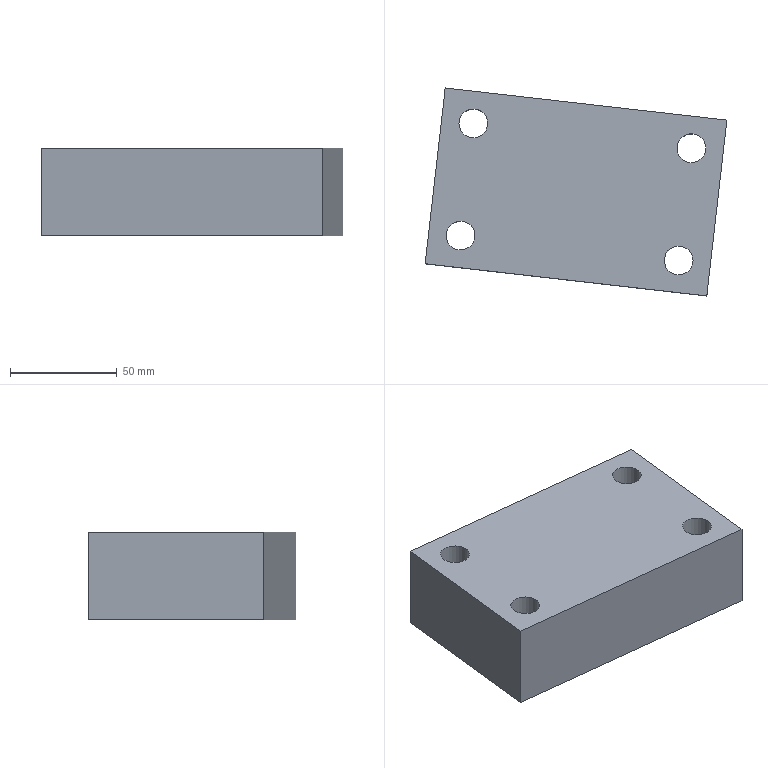Part | NX | features solid 2 | 1 solid | 18 faces | box 141.541 x 97.522 x 41 mm | volume 418863 mm3 | plane 10 | cylinder 8 | commonest cylinder face diameters 13.5 x4 20 x4
STEP:
#1=CARTESIAN_POINT('',(2413.748,-103.871,101.));
#2=VERTEX_POINT('',#1);
#3=CARTESIAN_POINT('',(2406.998,-103.871,101.));
#4=DIRECTION('',(0.,0.,-1.));
#5=DIRECTION('',(1.,0.,0.));
#6=AXIS2_PLACEMENT_3D('',#3,#4,#5);
#7=CIRCLE('',#6,6.75);
#8=EDGE_CURVE('',#2,#2,#7,.T.);
#9=ORIENTED_EDGE('',*,*,#8,.T.);
#10=EDGE_LOOP('',(#9));
#11=FACE_BOUND('',#10,.T.);
#12=CARTESIAN_POINT('',(2419.575,-52.73,101.));
#13=VERTEX_POINT('',#12);
#14=CARTESIAN_POINT('',(2412.998,-51.211,101.));
#15=DIRECTION('',(0.,0.,1.));
#16=DIRECTION('',(0.9744,-0.225,0.));
#17=AXIS2_PLACEMENT_3D('',#14,#15,#16);
#18=CIRCLE('',#17,6.75);
#19=EDGE_CURVE('',#13,#13,#18,.T.);
#20=ORIENTED_EDGE('',*,*,#19,.F.);
#21=EDGE_LOOP('',(#20));
#22=FACE_BOUND('',#21,.T.);
#23=CARTESIAN_POINT('',(2420.203,-120.472,101.));
#24=VERTEX_POINT('',#23);
#25=CARTESIAN_POINT('',(2288.058,-105.416,101.));
#26=VERTEX_POINT('',#25);
#27=CARTESIAN_POINT('',(2343.698,-111.756,101.));
#28=DIRECTION('',(-0.9936,0.1132,0.));
#29=VECTOR('',#28,1000.);
#30=LINE('',#27,#29);
#31=EDGE_CURVE('',#24,#26,#30,.T.);
#32=ORIENTED_EDGE('',*,*,#31,.F.);
#33=CARTESIAN_POINT('',(2429.599,-38.006,101.));
#34=VERTEX_POINT('',#33);
#35=CARTESIAN_POINT('',(2424.505,-82.717,101.));
#36=DIRECTION('',(-0.1132,-0.9936,0.));
#37=VECTOR('',#36,1000.);
#38=LINE('',#35,#37);
#39=EDGE_CURVE('',#34,#24,#38,.T.);
#40=ORIENTED_EDGE('',*,*,#39,.F.);
#41=CARTESIAN_POINT('',(2297.454,-22.95,101.));
#42=VERTEX_POINT('',#41);
#43=CARTESIAN_POINT('',(2353.094,-29.289,101.));
#44=DIRECTION('',(0.9936,-0.1132,0.));
#45=VECTOR('',#44,1000.);
#46=LINE('',#43,#45);
#47=EDGE_CURVE('',#42,#34,#46,.T.);
#48=ORIENTED_EDGE('',*,*,#47,.F.);
#49=CARTESIAN_POINT('',(2292.36,-67.661,101.));
#50=DIRECTION('',(0.1132,0.9936,0.));
#51=VECTOR('',#50,1000.);
#52=LINE('',#49,#51);
#53=EDGE_CURVE('',#26,#42,#52,.T.);
#54=ORIENTED_EDGE('',*,*,#53,.F.);
#55=EDGE_LOOP('',(#32,#40,#48,#54));
#56=FACE_BOUND('',#55,.T.);
#57=CARTESIAN_POINT('',(2298.083,-90.692,101.));
#58=VERTEX_POINT('',#57);
#59=CARTESIAN_POINT('',(2304.66,-92.211,101.));
#60=DIRECTION('',(0.,0.,1.));
#61=DIRECTION('',(-0.9744,0.225,0.));
#62=AXIS2_PLACEMENT_3D('',#59,#60,#61);
#63=CIRCLE('',#62,6.75);
#64=EDGE_CURVE('',#58,#58,#63,.T.);
#65=ORIENTED_EDGE('',*,*,#64,.F.);
#66=EDGE_LOOP('',(#65));
#67=FACE_BOUND('',#66,.T.);
#68=CARTESIAN_POINT('',(2303.91,-39.552,101.));
#69=VERTEX_POINT('',#68);
#70=CARTESIAN_POINT('',(2310.66,-39.552,101.));
#71=DIRECTION('',(0.,0.,-1.));
#72=DIRECTION('',(-1.,0.,0.));
#73=AXIS2_PLACEMENT_3D('',#70,#71,#72);
#74=CIRCLE('',#73,6.75);
#75=EDGE_CURVE('',#69,#69,#74,.T.);
#76=ORIENTED_EDGE('',*,*,#75,.T.);
#77=EDGE_LOOP('',(#76));
#78=FACE_BOUND('',#77,.T.);
#79=CARTESIAN_POINT('',(94.5,193.,101.));
#80=DIRECTION('',(0.,0.,1.));
#81=DIRECTION('',(-1.,0.,0.));
#82=AXIS2_PLACEMENT_3D('',#79,#80,#81);
#83=PLANE('',#82);
#84=ADVANCED_FACE('',(#11,#22,#56,#67,#78),#83,.T.);
#85=CARTESIAN_POINT('',(2416.998,-103.871,60.));
#86=VERTEX_POINT('',#85);
#87=CARTESIAN_POINT('',(2406.998,-103.871,60.));
#88=DIRECTION('',(0.,0.,1.));
#89=DIRECTION('',(1.,0.,0.));
#90=AXIS2_PLACEMENT_3D('',#87,#88,#89);
#91=CIRCLE('',#90,10.);
#92=EDGE_CURVE('',#86,#86,#91,.T.);
#93=ORIENTED_EDGE('',*,*,#92,.T.);
#94=EDGE_LOOP('',(#93));
#95=FACE_BOUND('',#94,.T.);
#96=CARTESIAN_POINT('',(2422.741,-53.461,60.));
#97=VERTEX_POINT('',#96);
#98=CARTESIAN_POINT('',(2412.998,-51.211,60.));
#99=DIRECTION('',(0.,0.,-1.));
#100=DIRECTION('',(0.9744,-0.225,0.));
#101=AXIS2_PLACEMENT_3D('',#98,#99,#100);
#102=CIRCLE('',#101,10.);
#103=EDGE_CURVE('',#97,#97,#102,.T.);
#104=ORIENTED_EDGE('',*,*,#103,.F.);
#105=EDGE_LOOP('',(#104));
#106=FACE_BOUND('',#105,.T.);
#107=CARTESIAN_POINT('',(2420.203,-120.472,60.));
#108=VERTEX_POINT('',#107);
#109=CARTESIAN_POINT('',(2429.599,-38.006,60.));
#110=VERTEX_POINT('',#109);
#111=CARTESIAN_POINT('',(2424.505,-82.717,60.));
#112=DIRECTION('',(0.1132,0.9936,0.));
#113=VECTOR('',#112,1000.);
#114=LINE('',#111,#113);
#115=EDGE_CURVE('',#108,#110,#114,.T.);
#116=ORIENTED_EDGE('',*,*,#115,.F.);
#117=CARTESIAN_POINT('',(2288.058,-105.416,60.));
#118=VERTEX_POINT('',#117);
#119=CARTESIAN_POINT('',(2343.698,-111.756,60.));
#120=DIRECTION('',(0.9936,-0.1132,0.));
#121=VECTOR('',#120,1000.);
#122=LINE('',#119,#121);
#123=EDGE_CURVE('',#118,#108,#122,.T.);
#124=ORIENTED_EDGE('',*,*,#123,.F.);
#125=CARTESIAN_POINT('',(2297.454,-22.95,60.));
#126=VERTEX_POINT('',#125);
#127=CARTESIAN_POINT('',(2292.36,-67.661,60.));
#128=DIRECTION('',(-0.1132,-0.9936,0.));
#129=VECTOR('',#128,1000.);
#130=LINE('',#127,#129);
#131=EDGE_CURVE('',#126,#118,#130,.T.);
#132=ORIENTED_EDGE('',*,*,#131,.F.);
#133=CARTESIAN_POINT('',(2353.094,-29.289,60.));
#134=DIRECTION('',(-0.9936,0.1132,0.));
#135=VECTOR('',#134,1000.);
#136=LINE('',#133,#135);
#137=EDGE_CURVE('',#110,#126,#136,.T.);
#138=ORIENTED_EDGE('',*,*,#137,.F.);
#139=EDGE_LOOP('',(#116,#124,#132,#138));
#140=FACE_BOUND('',#139,.T.);
#141=CARTESIAN_POINT('',(2294.916,-89.961,60.));
#142=VERTEX_POINT('',#141);
#143=CARTESIAN_POINT('',(2304.66,-92.211,60.));
#144=DIRECTION('',(0.,0.,-1.));
#145=DIRECTION('',(-0.9744,0.225,0.));
#146=AXIS2_PLACEMENT_3D('',#143,#144,#145);
#147=CIRCLE('',#146,10.);
#148=EDGE_CURVE('',#142,#142,#147,.T.);
#149=ORIENTED_EDGE('',*,*,#148,.F.);
#150=EDGE_LOOP('',(#149));
#151=FACE_BOUND('',#150,.T.);
#152=CARTESIAN_POINT('',(2300.66,-39.552,60.));
#153=VERTEX_POINT('',#152);
#154=CARTESIAN_POINT('',(2310.66,-39.552,60.));
#155=DIRECTION('',(0.,0.,1.));
#156=DIRECTION('',(-1.,0.,0.));
#157=AXIS2_PLACEMENT_3D('',#154,#155,#156);
#158=CIRCLE('',#157,10.);
#159=EDGE_CURVE('',#153,#153,#158,.T.);
#160=ORIENTED_EDGE('',*,*,#159,.T.);
#161=EDGE_LOOP('',(#160));
#162=FACE_BOUND('',#161,.T.);
#163=CARTESIAN_POINT('',(2470.641,-285.511,60.));
#164=DIRECTION('',(0.,0.,1.));
#165=DIRECTION('',(-1.,0.,0.));
#166=AXIS2_PLACEMENT_3D('',#163,#164,#165);
#167=PLANE('',#166);
#168=ADVANCED_FACE('',(#95,#106,#140,#151,#162),#167,.F.);
#169=CARTESIAN_POINT('',(2420.203,-120.472,-10.));
#170=DIRECTION('',(0.,0.,1.));
#171=VECTOR('',#170,1000.);
#172=LINE('',#169,#171);
#173=EDGE_CURVE('',#108,#24,#172,.T.);
#174=ORIENTED_EDGE('',*,*,#173,.T.);
#175=ORIENTED_EDGE('',*,*,#31,.T.);
#176=CARTESIAN_POINT('',(2288.058,-105.416,-10.));
#177=DIRECTION('',(0.,0.,1.));
#178=VECTOR('',#177,1000.);
#179=LINE('',#176,#178);
#180=EDGE_CURVE('',#118,#26,#179,.T.);
#181=ORIENTED_EDGE('',*,*,#180,.F.);
#182=ORIENTED_EDGE('',*,*,#123,.T.);
#183=EDGE_LOOP('',(#174,#175,#181,#182));
#184=FACE_BOUND('',#183,.T.);
#185=CARTESIAN_POINT('',(2343.698,-111.756,-10.));
#186=DIRECTION('',(-0.1132,-0.9936,0.));
#187=DIRECTION('',(-0.9936,0.1132,0.));
#188=AXIS2_PLACEMENT_3D('',#185,#186,#187);
#189=PLANE('',#188);
#190=ADVANCED_FACE('',(#184),#189,.T.);
#191=ORIENTED_EDGE('',*,*,#180,.T.);
#192=ORIENTED_EDGE('',*,*,#53,.T.);
#193=CARTESIAN_POINT('',(2297.454,-22.95,-10.));
#194=DIRECTION('',(0.,0.,1.));
#195=VECTOR('',#194,1000.);
#196=LINE('',#193,#195);
#197=EDGE_CURVE('',#126,#42,#196,.T.);
#198=ORIENTED_EDGE('',*,*,#197,.F.);
#199=ORIENTED_EDGE('',*,*,#131,.T.);
#200=EDGE_LOOP('',(#191,#192,#198,#199));
#201=FACE_BOUND('',#200,.T.);
#202=CARTESIAN_POINT('',(2292.36,-67.661,-10.));
#203=DIRECTION('',(-0.9936,0.1132,0.));
#204=DIRECTION('',(0.1132,0.9936,0.));
#205=AXIS2_PLACEMENT_3D('',#202,#203,#204);
#206=PLANE('',#205);
#207=ADVANCED_FACE('',(#201),#206,.T.);
#208=ORIENTED_EDGE('',*,*,#197,.T.);
#209=ORIENTED_EDGE('',*,*,#47,.T.);
#210=CARTESIAN_POINT('',(2429.599,-38.006,-10.));
#211=DIRECTION('',(0.,0.,1.));
#212=VECTOR('',#211,1000.);
#213=LINE('',#210,#212);
#214=EDGE_CURVE('',#110,#34,#213,.T.);
#215=ORIENTED_EDGE('',*,*,#214,.F.);
#216=ORIENTED_EDGE('',*,*,#137,.T.);
#217=EDGE_LOOP('',(#208,#209,#215,#216));
#218=FACE_BOUND('',#217,.T.);
#219=CARTESIAN_POINT('',(2353.094,-29.289,-10.));
#220=DIRECTION('',(0.1132,0.9936,0.));
#221=DIRECTION('',(0.9936,-0.1132,0.));
#222=AXIS2_PLACEMENT_3D('',#219,#220,#221);
#223=PLANE('',#222);
#224=ADVANCED_FACE('',(#218),#223,.T.);
#225=ORIENTED_EDGE('',*,*,#115,.T.);
#226=ORIENTED_EDGE('',*,*,#214,.T.);
#227=ORIENTED_EDGE('',*,*,#39,.T.);
#228=ORIENTED_EDGE('',*,*,#173,.F.);
#229=EDGE_LOOP('',(#225,#226,#227,#228));
#230=FACE_BOUND('',#229,.T.);
#231=CARTESIAN_POINT('',(2424.505,-82.717,-10.));
#232=DIRECTION('',(0.9936,-0.1132,0.));
#233=DIRECTION('',(-0.1132,-0.9936,0.));
#234=AXIS2_PLACEMENT_3D('',#231,#232,#233);
#235=PLANE('',#234);
#236=ADVANCED_FACE('',(#230),#235,.T.);
#237=CARTESIAN_POINT('',(2419.575,-52.73,75.));
#238=VERTEX_POINT('',#237);
#239=CARTESIAN_POINT('',(2412.998,-51.211,75.));
#240=DIRECTION('',(0.,0.,-1.));
#241=DIRECTION('',(0.9744,-0.225,0.));
#242=AXIS2_PLACEMENT_3D('',#239,#240,#241);
#243=CIRCLE('',#242,6.75);
#244=EDGE_CURVE('',#238,#238,#243,.T.);
#245=ORIENTED_EDGE('',*,*,#244,.T.);
#246=EDGE_LOOP('',(#245));
#247=FACE_BOUND('',#246,.T.);
#248=ORIENTED_EDGE('',*,*,#19,.T.);
#249=EDGE_LOOP('',(#248));
#250=FACE_BOUND('',#249,.T.);
#251=CARTESIAN_POINT('',(2412.998,-51.211,60.));
#252=DIRECTION('',(0.,0.,1.));
#253=DIRECTION('',(-0.9744,0.225,0.));
#254=AXIS2_PLACEMENT_3D('',#251,#252,#253);
#255=CYLINDRICAL_SURFACE('',#254,6.75);
#256=ADVANCED_FACE('',(#247,#250),#255,.F.);
#257=ORIENTED_EDGE('',*,*,#244,.F.);
#258=EDGE_LOOP('',(#257));
#259=FACE_BOUND('',#258,.T.);
#260=CARTESIAN_POINT('',(2422.741,-53.461,75.));
#261=VERTEX_POINT('',#260);
#262=CARTESIAN_POINT('',(2412.998,-51.211,75.));
#263=DIRECTION('',(0.,0.,-1.));
#264=DIRECTION('',(0.9744,-0.225,0.));
#265=AXIS2_PLACEMENT_3D('',#262,#263,#264);
#266=CIRCLE('',#265,10.);
#267=EDGE_CURVE('',#261,#261,#266,.T.);
#268=ORIENTED_EDGE('',*,*,#267,.T.);
#269=EDGE_LOOP('',(#268));
#270=FACE_BOUND('',#269,.T.);
#271=CARTESIAN_POINT('',(2412.998,-51.211,75.));
#272=DIRECTION('',(0.,0.,1.));
#273=DIRECTION('',(-0.9744,0.225,0.));
#274=AXIS2_PLACEMENT_3D('',#271,#272,#273);
#275=PLANE('',#274);
#276=ADVANCED_FACE('',(#259,#270),#275,.F.);
#277=ORIENTED_EDGE('',*,*,#267,.F.);
#278=EDGE_LOOP('',(#277));
#279=FACE_BOUND('',#278,.T.);
#280=ORIENTED_EDGE('',*,*,#103,.T.);
#281=EDGE_LOOP('',(#280));
#282=FACE_BOUND('',#281,.T.);
#283=CARTESIAN_POINT('',(2412.998,-51.211,60.));
#284=DIRECTION('',(0.,0.,1.));
#285=DIRECTION('',(-0.9744,0.225,0.));
#286=AXIS2_PLACEMENT_3D('',#283,#284,#285);
#287=CYLINDRICAL_SURFACE('',#286,10.);
#288=ADVANCED_FACE('',(#279,#282),#287,.F.);
#289=CARTESIAN_POINT('',(2413.748,-103.871,75.));
#290=VERTEX_POINT('',#289);
#291=CARTESIAN_POINT('',(2406.998,-103.871,75.));
#292=DIRECTION('',(0.,0.,1.));
#293=DIRECTION('',(1.,0.,0.));
#294=AXIS2_PLACEMENT_3D('',#291,#292,#293);
#295=CIRCLE('',#294,6.75);
#296=EDGE_CURVE('',#290,#290,#295,.T.);
#297=ORIENTED_EDGE('',*,*,#296,.F.);
#298=EDGE_LOOP('',(#297));
#299=FACE_BOUND('',#298,.T.);
#300=ORIENTED_EDGE('',*,*,#8,.F.);
#301=EDGE_LOOP('',(#300));
#302=FACE_BOUND('',#301,.T.);
#303=CARTESIAN_POINT('',(2406.998,-103.871,60.));
#304=DIRECTION('',(0.,0.,1.));
#305=DIRECTION('',(-1.,0.,0.));
#306=AXIS2_PLACEMENT_3D('',#303,#304,#305);
#307=CYLINDRICAL_SURFACE('',#306,6.75);
#308=ADVANCED_FACE('',(#299,#302),#307,.F.);
#309=ORIENTED_EDGE('',*,*,#296,.T.);
#310=EDGE_LOOP('',(#309));
#311=FACE_BOUND('',#310,.T.);
#312=CARTESIAN_POINT('',(2416.998,-103.871,75.));
#313=VERTEX_POINT('',#312);
#314=CARTESIAN_POINT('',(2406.998,-103.871,75.));
#315=DIRECTION('',(0.,0.,1.));
#316=DIRECTION('',(1.,0.,0.));
#317=AXIS2_PLACEMENT_3D('',#314,#315,#316);
#318=CIRCLE('',#317,10.);
#319=EDGE_CURVE('',#313,#313,#318,.T.);
#320=ORIENTED_EDGE('',*,*,#319,.F.);
#321=EDGE_LOOP('',(#320));
#322=FACE_BOUND('',#321,.T.);
#323=CARTESIAN_POINT('',(2405.073,-120.761,75.));
#324=DIRECTION('',(0.,0.,1.));
#325=DIRECTION('',(-1.,0.,0.));
#326=AXIS2_PLACEMENT_3D('',#323,#324,#325);
#327=PLANE('',#326);
#328=ADVANCED_FACE('',(#311,#322),#327,.F.);
#329=ORIENTED_EDGE('',*,*,#319,.T.);
#330=EDGE_LOOP('',(#329));
#331=FACE_BOUND('',#330,.T.);
#332=ORIENTED_EDGE('',*,*,#92,.F.);
#333=EDGE_LOOP('',(#332));
#334=FACE_BOUND('',#333,.T.);
#335=CARTESIAN_POINT('',(2406.998,-103.871,60.));
#336=DIRECTION('',(0.,0.,1.));
#337=DIRECTION('',(-1.,0.,0.));
#338=AXIS2_PLACEMENT_3D('',#335,#336,#337);
#339=CYLINDRICAL_SURFACE('',#338,10.);
#340=ADVANCED_FACE('',(#331,#334),#339,.F.);
#341=CARTESIAN_POINT('',(2298.083,-90.692,75.));
#342=VERTEX_POINT('',#341);
#343=CARTESIAN_POINT('',(2304.66,-92.211,75.));
#344=DIRECTION('',(0.,0.,-1.));
#345=DIRECTION('',(-0.9744,0.225,0.));
#346=AXIS2_PLACEMENT_3D('',#343,#344,#345);
#347=CIRCLE('',#346,6.75);
#348=EDGE_CURVE('',#342,#342,#347,.T.);
#349=ORIENTED_EDGE('',*,*,#348,.T.);
#350=EDGE_LOOP('',(#349));
#351=FACE_BOUND('',#350,.T.);
#352=ORIENTED_EDGE('',*,*,#64,.T.);
#353=EDGE_LOOP('',(#352));
#354=FACE_BOUND('',#353,.T.);
#355=CARTESIAN_POINT('',(2304.66,-92.211,60.));
#356=DIRECTION('',(0.,0.,1.));
#357=DIRECTION('',(0.9744,-0.225,0.));
#358=AXIS2_PLACEMENT_3D('',#355,#356,#357);
#359=CYLINDRICAL_SURFACE('',#358,6.75);
#360=ADVANCED_FACE('',(#351,#354),#359,.F.);
#361=ORIENTED_EDGE('',*,*,#348,.F.);
#362=EDGE_LOOP('',(#361));
#363=FACE_BOUND('',#362,.T.);
#364=CARTESIAN_POINT('',(2294.916,-89.961,75.));
#365=VERTEX_POINT('',#364);
#366=CARTESIAN_POINT('',(2304.66,-92.211,75.));
#367=DIRECTION('',(0.,0.,-1.));
#368=DIRECTION('',(-0.9744,0.225,0.));
#369=AXIS2_PLACEMENT_3D('',#366,#367,#368);
#370=CIRCLE('',#369,10.);
#371=EDGE_CURVE('',#365,#365,#370,.T.);
#372=ORIENTED_EDGE('',*,*,#371,.T.);
#373=EDGE_LOOP('',(#372));
#374=FACE_BOUND('',#373,.T.);
#375=CARTESIAN_POINT('',(2302.735,-109.102,75.));
#376=DIRECTION('',(0.,0.,1.));
#377=DIRECTION('',(0.9744,-0.225,0.));
#378=AXIS2_PLACEMENT_3D('',#375,#376,#377);
#379=PLANE('',#378);
#380=ADVANCED_FACE('',(#363,#374),#379,.F.);
#381=ORIENTED_EDGE('',*,*,#371,.F.);
#382=EDGE_LOOP('',(#381));
#383=FACE_BOUND('',#382,.T.);
#384=ORIENTED_EDGE('',*,*,#148,.T.);
#385=EDGE_LOOP('',(#384));
#386=FACE_BOUND('',#385,.T.);
#387=CARTESIAN_POINT('',(2304.66,-92.211,60.));
#388=DIRECTION('',(0.,0.,1.));
#389=DIRECTION('',(0.9744,-0.225,0.));
#390=AXIS2_PLACEMENT_3D('',#387,#388,#389);
#391=CYLINDRICAL_SURFACE('',#390,10.);
#392=ADVANCED_FACE('',(#383,#386),#391,.F.);
#393=CARTESIAN_POINT('',(2303.91,-39.552,75.));
#394=VERTEX_POINT('',#393);
#395=CARTESIAN_POINT('',(2310.66,-39.552,75.));
#396=DIRECTION('',(0.,0.,1.));
#397=DIRECTION('',(-1.,0.,0.));
#398=AXIS2_PLACEMENT_3D('',#395,#396,#397);
#399=CIRCLE('',#398,6.75);
#400=EDGE_CURVE('',#394,#394,#399,.T.);
#401=ORIENTED_EDGE('',*,*,#400,.F.);
#402=EDGE_LOOP('',(#401));
#403=FACE_BOUND('',#402,.T.);
#404=ORIENTED_EDGE('',*,*,#75,.F.);
#405=EDGE_LOOP('',(#404));
#406=FACE_BOUND('',#405,.T.);
#407=CARTESIAN_POINT('',(2310.66,-39.552,60.));
#408=DIRECTION('',(0.,0.,1.));
#409=DIRECTION('',(1.,0.,0.));
#410=AXIS2_PLACEMENT_3D('',#407,#408,#409);
#411=CYLINDRICAL_SURFACE('',#410,6.75);
#412=ADVANCED_FACE('',(#403,#406),#411,.F.);
#413=ORIENTED_EDGE('',*,*,#400,.T.);
#414=EDGE_LOOP('',(#413));
#415=FACE_BOUND('',#414,.T.);
#416=CARTESIAN_POINT('',(2300.66,-39.552,75.));
#417=VERTEX_POINT('',#416);
#418=CARTESIAN_POINT('',(2310.66,-39.552,75.));
#419=DIRECTION('',(0.,0.,1.));
#420=DIRECTION('',(-1.,0.,0.));
#421=AXIS2_PLACEMENT_3D('',#418,#419,#420);
#422=CIRCLE('',#421,10.);
#423=EDGE_CURVE('',#417,#417,#422,.T.);
#424=ORIENTED_EDGE('',*,*,#423,.F.);
#425=EDGE_LOOP('',(#424));
#426=FACE_BOUND('',#425,.T.);
#427=CARTESIAN_POINT('',(2310.66,-39.552,75.));
#428=DIRECTION('',(0.,0.,1.));
#429=DIRECTION('',(1.,0.,0.));
#430=AXIS2_PLACEMENT_3D('',#427,#428,#429);
#431=PLANE('',#430);
#432=ADVANCED_FACE('',(#415,#426),#431,.F.);
#433=ORIENTED_EDGE('',*,*,#423,.T.);
#434=EDGE_LOOP('',(#433));
#435=FACE_BOUND('',#434,.T.);
#436=ORIENTED_EDGE('',*,*,#159,.F.);
#437=EDGE_LOOP('',(#436));
#438=FACE_BOUND('',#437,.T.);
#439=CARTESIAN_POINT('',(2310.66,-39.552,60.));
#440=DIRECTION('',(0.,0.,1.));
#441=DIRECTION('',(1.,0.,0.));
#442=AXIS2_PLACEMENT_3D('',#439,#440,#441);
#443=CYLINDRICAL_SURFACE('',#442,10.);
#444=ADVANCED_FACE('',(#435,#438),#443,.F.);
#445=CLOSED_SHELL('',(#84,#168,#190,#207,#224,#236,#256,#276,#288,#308,#328,#340,#360,#380,#392,#412,#432,#444));
#446=MANIFOLD_SOLID_BREP('',#445);
#447=(LENGTH_UNIT()NAMED_UNIT(*)SI_UNIT(.MILLI.,.METRE.));
#448=UNCERTAINTY_MEASURE_WITH_UNIT(LENGTH_MEASURE(0.00001),#447,'','');
#449=(NAMED_UNIT(*)PLANE_ANGLE_UNIT()SI_UNIT($,.RADIAN.));
#450=(NAMED_UNIT(*)SI_UNIT($,.STERADIAN.)SOLID_ANGLE_UNIT());
#451=(GEOMETRIC_REPRESENTATION_CONTEXT(3)GLOBAL_UNCERTAINTY_ASSIGNED_CONTEXT((#448))GLOBAL_UNIT_ASSIGNED_CONTEXT((#447,#449,#450))REPRESENTATION_CONTEXT('',''));
#452=ADVANCED_BREP_SHAPE_REPRESENTATION('',(#446),#451);